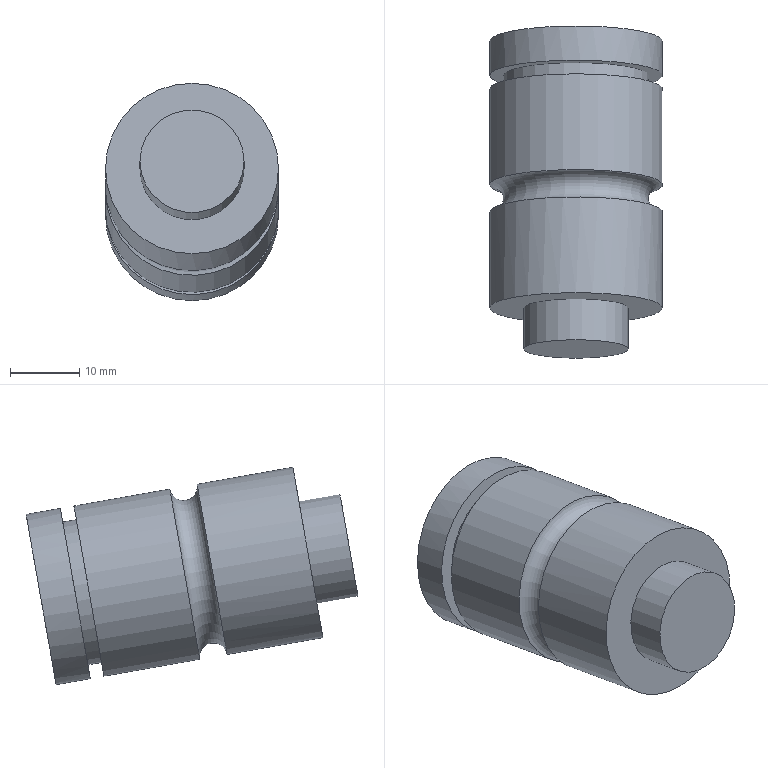Part | NX | features MAIN_BODY 2 | 1 solid | 11 faces | box 24.9 x 47.781 x 31.294 mm | volume 19306 mm3 | cylinder 5 | plane 5 | torus 1 | commonest cylinder face diameters 24.9 x3 15 x1 20.9 x1
STEP:
#1=CARTESIAN_POINT('',(-1020.95,-797.245,42.626));
#2=VERTEX_POINT('',#1);
#3=CARTESIAN_POINT('',(-1008.5,-797.245,42.626));
#4=DIRECTION('',(0.,0.9848,-0.1736));
#5=DIRECTION('',(-1.,0.,0.));
#6=AXIS2_PLACEMENT_3D('',#3,#4,#5);
#7=CIRCLE('',#6,12.45);
#8=EDGE_CURVE('',#2,#2,#7,.F.);
#9=ORIENTED_EDGE('',*,*,#8,.T.);
#10=EDGE_LOOP('',(#9));
#11=FACE_BOUND('',#10,.T.);
#12=CARTESIAN_POINT('',(-1020.95,-811.032,45.057));
#13=VERTEX_POINT('',#12);
#14=CARTESIAN_POINT('',(-1008.5,-811.032,45.057));
#15=DIRECTION('',(0.,0.9848,-0.1736));
#16=DIRECTION('',(-1.,0.,0.));
#17=AXIS2_PLACEMENT_3D('',#14,#15,#16);
#18=CIRCLE('',#17,12.45);
#19=EDGE_CURVE('',#13,#13,#18,.T.);
#20=ORIENTED_EDGE('',*,*,#19,.T.);
#21=EDGE_LOOP('',(#20));
#22=FACE_BOUND('',#21,.T.);
#23=CARTESIAN_POINT('',(-1008.5,-828.759,48.183));
#24=DIRECTION('',(0.,0.9848,-0.1736));
#25=DIRECTION('',(-1.,0.,0.));
#26=AXIS2_PLACEMENT_3D('',#23,#24,#25);
#27=CYLINDRICAL_SURFACE('',#26,12.45);
#28=ADVANCED_FACE('',(#11,#22),#27,.T.);
#29=CARTESIAN_POINT('',(-996.05,-828.759,48.183));
#30=VERTEX_POINT('',#29);
#31=CARTESIAN_POINT('',(-1008.5,-828.759,48.183));
#32=DIRECTION('',(0.,-0.9848,0.1736));
#33=DIRECTION('',(1.,0.,0.));
#34=AXIS2_PLACEMENT_3D('',#31,#32,#33);
#35=CIRCLE('',#34,12.45);
#36=EDGE_CURVE('',#30,#30,#35,.T.);
#37=ORIENTED_EDGE('',*,*,#36,.T.);
#38=EDGE_LOOP('',(#37));
#39=FACE_BOUND('',#38,.T.);
#40=CARTESIAN_POINT('',(-1001.,-828.759,48.183));
#41=VERTEX_POINT('',#40);
#42=CARTESIAN_POINT('',(-1008.5,-828.759,48.183));
#43=DIRECTION('',(0.,-0.9848,0.1736));
#44=DIRECTION('',(1.,0.,0.));
#45=AXIS2_PLACEMENT_3D('',#42,#43,#44);
#46=CIRCLE('',#45,7.5);
#47=EDGE_CURVE('',#41,#41,#46,.T.);
#48=ORIENTED_EDGE('',*,*,#47,.F.);
#49=EDGE_LOOP('',(#48));
#50=FACE_BOUND('',#49,.T.);
#51=CARTESIAN_POINT('',(-1008.5,-828.759,48.183));
#52=DIRECTION('',(0.,-0.9848,0.1736));
#53=DIRECTION('',(1.,0.,0.));
#54=AXIS2_PLACEMENT_3D('',#51,#52,#53);
#55=PLANE('',#54);
#56=ADVANCED_FACE('',(#39,#50),#55,.T.);
#57=CARTESIAN_POINT('',(-1020.95,-814.972,45.752));
#58=VERTEX_POINT('',#57);
#59=CARTESIAN_POINT('',(-1008.5,-814.972,45.752));
#60=DIRECTION('',(0.,0.9848,-0.1736));
#61=DIRECTION('',(-1.,0.,0.));
#62=AXIS2_PLACEMENT_3D('',#59,#60,#61);
#63=CIRCLE('',#62,12.45);
#64=EDGE_CURVE('',#58,#58,#63,.F.);
#65=ORIENTED_EDGE('',*,*,#64,.T.);
#66=EDGE_LOOP('',(#65));
#67=FACE_BOUND('',#66,.T.);
#68=ORIENTED_EDGE('',*,*,#36,.F.);
#69=EDGE_LOOP('',(#68));
#70=FACE_BOUND('',#69,.T.);
#71=CARTESIAN_POINT('',(-1008.5,-828.759,48.183));
#72=DIRECTION('',(0.,0.9848,-0.1736));
#73=DIRECTION('',(-1.,0.,0.));
#74=AXIS2_PLACEMENT_3D('',#71,#72,#73);
#75=CYLINDRICAL_SURFACE('',#74,12.45);
#76=ADVANCED_FACE('',(#67,#70),#75,.T.);
#77=ORIENTED_EDGE('',*,*,#47,.T.);
#78=EDGE_LOOP('',(#77));
#79=FACE_BOUND('',#78,.T.);
#80=CARTESIAN_POINT('',(-1001.,-834.668,49.225));
#81=VERTEX_POINT('',#80);
#82=CARTESIAN_POINT('',(-1008.5,-834.668,49.225));
#83=DIRECTION('',(0.,-0.9848,0.1736));
#84=DIRECTION('',(1.,0.,0.));
#85=AXIS2_PLACEMENT_3D('',#82,#83,#84);
#86=CIRCLE('',#85,7.5);
#87=EDGE_CURVE('',#81,#81,#86,.T.);
#88=ORIENTED_EDGE('',*,*,#87,.F.);
#89=EDGE_LOOP('',(#88));
#90=FACE_BOUND('',#89,.T.);
#91=CARTESIAN_POINT('',(-1008.5,-829.744,48.357));
#92=DIRECTION('',(0.,0.9848,-0.1736));
#93=DIRECTION('',(-1.,0.,0.));
#94=AXIS2_PLACEMENT_3D('',#91,#92,#93);
#95=CYLINDRICAL_SURFACE('',#94,7.5);
#96=ADVANCED_FACE('',(#79,#90),#95,.T.);
#97=ORIENTED_EDGE('',*,*,#64,.F.);
#98=EDGE_LOOP('',(#97));
#99=FACE_BOUND('',#98,.T.);
#100=ORIENTED_EDGE('',*,*,#19,.F.);
#101=EDGE_LOOP('',(#100));
#102=FACE_BOUND('',#101,.T.);
#103=CARTESIAN_POINT('',(-1008.5,-813.002,45.405));
#104=DIRECTION('',(0.,0.9848,-0.1736));
#105=DIRECTION('',(-1.,0.,0.));
#106=AXIS2_PLACEMENT_3D('',#103,#104,#105);
#107=TOROIDAL_SURFACE('',#106,12.45,2.);
#108=ADVANCED_FACE('',(#99,#102),#107,.F.);
#109=CARTESIAN_POINT('',(-998.05,-797.245,42.626));
#110=VERTEX_POINT('',#109);
#111=CARTESIAN_POINT('',(-1008.5,-797.245,42.626));
#112=DIRECTION('',(0.,-0.9848,0.1736));
#113=DIRECTION('',(1.,0.,0.));
#114=AXIS2_PLACEMENT_3D('',#111,#112,#113);
#115=CIRCLE('',#114,10.45);
#116=EDGE_CURVE('',#110,#110,#115,.T.);
#117=ORIENTED_EDGE('',*,*,#116,.T.);
#118=EDGE_LOOP('',(#117));
#119=FACE_BOUND('',#118,.T.);
#120=ORIENTED_EDGE('',*,*,#8,.F.);
#121=EDGE_LOOP('',(#120));
#122=FACE_BOUND('',#121,.T.);
#123=CARTESIAN_POINT('',(-1008.5,-797.245,42.626));
#124=DIRECTION('',(0.,0.9848,-0.1736));
#125=DIRECTION('',(-1.,0.,0.));
#126=AXIS2_PLACEMENT_3D('',#123,#124,#125);
#127=PLANE('',#126);
#128=ADVANCED_FACE('',(#119,#122),#127,.T.);
#129=CARTESIAN_POINT('',(-998.05,-795.275,42.279));
#130=VERTEX_POINT('',#129);
#131=CARTESIAN_POINT('',(-1008.5,-795.275,42.279));
#132=DIRECTION('',(0.,-0.9848,0.1736));
#133=DIRECTION('',(1.,0.,0.));
#134=AXIS2_PLACEMENT_3D('',#131,#132,#133);
#135=CIRCLE('',#134,10.45);
#136=EDGE_CURVE('',#130,#130,#135,.T.);
#137=ORIENTED_EDGE('',*,*,#136,.F.);
#138=EDGE_LOOP('',(#137));
#139=FACE_BOUND('',#138,.T.);
#140=CARTESIAN_POINT('',(-1020.95,-795.275,42.279));
#141=VERTEX_POINT('',#140);
#142=CARTESIAN_POINT('',(-1008.5,-795.275,42.279));
#143=DIRECTION('',(0.,0.9848,-0.1736));
#144=DIRECTION('',(-1.,0.,0.));
#145=AXIS2_PLACEMENT_3D('',#142,#143,#144);
#146=CIRCLE('',#145,12.45);
#147=EDGE_CURVE('',#141,#141,#146,.T.);
#148=ORIENTED_EDGE('',*,*,#147,.F.);
#149=EDGE_LOOP('',(#148));
#150=FACE_BOUND('',#149,.T.);
#151=CARTESIAN_POINT('',(-1008.5,-795.275,42.279));
#152=DIRECTION('',(0.,0.9848,-0.1736));
#153=DIRECTION('',(-1.,0.,0.));
#154=AXIS2_PLACEMENT_3D('',#151,#152,#153);
#155=PLANE('',#154);
#156=ADVANCED_FACE('',(#139,#150),#155,.F.);
#157=ORIENTED_EDGE('',*,*,#116,.F.);
#158=EDGE_LOOP('',(#157));
#159=FACE_BOUND('',#158,.T.);
#160=ORIENTED_EDGE('',*,*,#136,.T.);
#161=EDGE_LOOP('',(#160));
#162=FACE_BOUND('',#161,.T.);
#163=CARTESIAN_POINT('',(-1008.5,-795.275,42.279));
#164=DIRECTION('',(0.,-0.9848,0.1736));
#165=DIRECTION('',(1.,0.,0.));
#166=AXIS2_PLACEMENT_3D('',#163,#164,#165);
#167=CYLINDRICAL_SURFACE('',#166,10.45);
#168=ADVANCED_FACE('',(#159,#162),#167,.T.);
#169=CARTESIAN_POINT('',(-996.05,-790.351,41.411));
#170=VERTEX_POINT('',#169);
#171=CARTESIAN_POINT('',(-1008.5,-790.351,41.411));
#172=DIRECTION('',(0.,-0.9848,0.1736));
#173=DIRECTION('',(1.,0.,0.));
#174=AXIS2_PLACEMENT_3D('',#171,#172,#173);
#175=CIRCLE('',#174,12.45);
#176=EDGE_CURVE('',#170,#170,#175,.T.);
#177=ORIENTED_EDGE('',*,*,#176,.F.);
#178=EDGE_LOOP('',(#177));
#179=FACE_BOUND('',#178,.T.);
#180=CARTESIAN_POINT('',(-1008.5,-790.351,41.411));
#181=DIRECTION('',(0.,-0.9848,0.1736));
#182=DIRECTION('',(1.,0.,0.));
#183=AXIS2_PLACEMENT_3D('',#180,#181,#182);
#184=PLANE('',#183);
#185=ADVANCED_FACE('',(#179),#184,.F.);
#186=ORIENTED_EDGE('',*,*,#147,.T.);
#187=EDGE_LOOP('',(#186));
#188=FACE_BOUND('',#187,.T.);
#189=ORIENTED_EDGE('',*,*,#176,.T.);
#190=EDGE_LOOP('',(#189));
#191=FACE_BOUND('',#190,.T.);
#192=CARTESIAN_POINT('',(-1008.5,-828.759,48.183));
#193=DIRECTION('',(0.,0.9848,-0.1736));
#194=DIRECTION('',(-1.,0.,0.));
#195=AXIS2_PLACEMENT_3D('',#192,#193,#194);
#196=CYLINDRICAL_SURFACE('',#195,12.45);
#197=ADVANCED_FACE('',(#188,#191),#196,.T.);
#198=ORIENTED_EDGE('',*,*,#87,.T.);
#199=EDGE_LOOP('',(#198));
#200=FACE_BOUND('',#199,.T.);
#201=CARTESIAN_POINT('',(-1008.5,-834.668,49.225));
#202=DIRECTION('',(0.,-0.9848,0.1736));
#203=DIRECTION('',(1.,0.,0.));
#204=AXIS2_PLACEMENT_3D('',#201,#202,#203);
#205=PLANE('',#204);
#206=ADVANCED_FACE('',(#200),#205,.T.);
#207=CLOSED_SHELL('',(#28,#56,#76,#96,#108,#128,#156,#168,#185,#197,#206));
#208=MANIFOLD_SOLID_BREP('',#207);
#209=(LENGTH_UNIT()NAMED_UNIT(*)SI_UNIT(.MILLI.,.METRE.));
#210=UNCERTAINTY_MEASURE_WITH_UNIT(LENGTH_MEASURE(0.00001),#209,'','');
#211=(NAMED_UNIT(*)PLANE_ANGLE_UNIT()SI_UNIT($,.RADIAN.));
#212=(NAMED_UNIT(*)SI_UNIT($,.STERADIAN.)SOLID_ANGLE_UNIT());
#213=(GEOMETRIC_REPRESENTATION_CONTEXT(3)GLOBAL_UNCERTAINTY_ASSIGNED_CONTEXT((#210))GLOBAL_UNIT_ASSIGNED_CONTEXT((#209,#211,#212))REPRESENTATION_CONTEXT('',''));
#214=ADVANCED_BREP_SHAPE_REPRESENTATION('',(#208),#213);